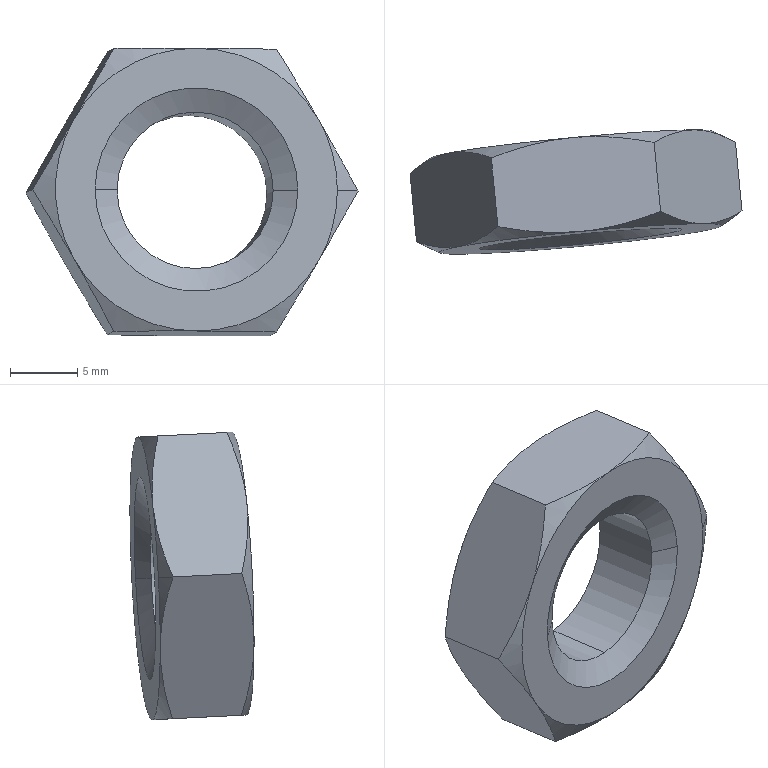Part | SolidWorks | features BaseBody 1 | 1 solid | 28 faces | box 24.623 x 9.204 x 21.336 mm | volume 1841 mm3 | cone 18 | plane 8 | cylinder 2 | commonest cylinder face diameters 11.62 x2
STEP:
#1=CARTESIAN_POINT('',(1944.046,536.426,848.503));
#2=VERTEX_POINT('',#1);
#3=CARTESIAN_POINT('',(1945.447,536.291,843.253));
#4=VERTEX_POINT('',#3);
#5=CARTESIAN_POINT('',(1934.993,535.304,843.303));
#6=DIRECTION('',(-0.09408,0.9943,-0.05066));
#7=DIRECTION('',(0.8622,0.1068,0.4952));
#8=AXIS2_PLACEMENT_3D('',#5,#6,#7);
#9=CIRCLE('',#8,10.5);
#10=EDGE_CURVE('',#2,#4,#9,.T.);
#11=ORIENTED_EDGE('',*,*,#10,.T.);
#12=CARTESIAN_POINT('',(1946.976,537.376,843.198));
#13=VERTEX_POINT('',#12);
#14=CARTESIAN_POINT('',(1946.211,536.833,843.226));
#15=DIRECTION('',(0.8151,0.5785,-0.02947));
#16=VECTOR('',#15,1000.);
#17=LINE('',#14,#16);
#18=EDGE_CURVE('',#4,#13,#17,.T.);
#19=ORIENTED_EDGE('',*,*,#18,.T.);
#20=CARTESIAN_POINT('',(1944.046,536.426,848.503));
#21=CARTESIAN_POINT('',(1944.561,536.429,847.606));
#22=CARTESIAN_POINT('',(1945.061,536.521,846.716));
#23=CARTESIAN_POINT('',(1946.035,536.851,844.949));
#24=CARTESIAN_POINT('',(1946.51,537.089,844.071));
#25=CARTESIAN_POINT('',(1946.976,537.376,843.198));
#26=B_SPLINE_CURVE_WITH_KNOTS('',3,(#20,#21,#22,#23,#24,#25),.UNSPECIFIED.,.F.,.F.,(4,2,4),(0.,0.003067,0.006134),.UNSPECIFIED.);
#27=EDGE_CURVE('',#2,#13,#26,.T.);
#28=ORIENTED_EDGE('',*,*,#27,.F.);
#29=EDGE_LOOP('',(#11,#19,#28));
#30=FACE_OUTER_BOUND('',#29,.T.);
#31=CARTESIAN_POINT('',(1934.949,535.77,843.28));
#32=DIRECTION('',(-0.09408,0.9943,-0.05066));
#33=DIRECTION('',(0.9956,0.09396,-0.004782));
#34=AXIS2_PLACEMENT_3D('',#31,#32,#33);
#35=CONICAL_SURFACE('',#34,11.312,1.047);
#36=ADVANCED_FACE('',(#30),#35,.T.);
#37=CARTESIAN_POINT('',(1925.282,541.677,848.235));
#38=VERTEX_POINT('',#37);
#39=CARTESIAN_POINT('',(1923.881,541.278,842.999));
#40=VERTEX_POINT('',#39);
#41=CARTESIAN_POINT('',(1934.335,542.264,842.949));
#42=DIRECTION('',(0.09408,-0.9943,0.05066));
#43=DIRECTION('',(-0.8622,-0.05593,0.5035));
#44=AXIS2_PLACEMENT_3D('',#41,#42,#43);
#45=CIRCLE('',#44,10.5);
#46=EDGE_CURVE('',#38,#40,#45,.T.);
#47=ORIENTED_EDGE('',*,*,#46,.T.);
#48=CARTESIAN_POINT('',(1922.352,540.193,843.054));
#49=VERTEX_POINT('',#48);
#50=CARTESIAN_POINT('',(1923.117,540.735,843.027));
#51=DIRECTION('',(-0.8151,-0.5785,0.02947));
#52=VECTOR('',#51,1000.);
#53=LINE('',#50,#52);
#54=EDGE_CURVE('',#40,#49,#53,.T.);
#55=ORIENTED_EDGE('',*,*,#54,.T.);
#56=CARTESIAN_POINT('',(1922.352,540.193,843.054));
#57=CARTESIAN_POINT('',(1922.818,540.567,843.894));
#58=CARTESIAN_POINT('',(1923.293,540.892,844.743));
#59=CARTESIAN_POINT('',(1924.267,541.401,846.467));
#60=CARTESIAN_POINT('',(1924.767,541.583,847.343));
#61=CARTESIAN_POINT('',(1925.282,541.677,848.235));
#62=B_SPLINE_CURVE_WITH_KNOTS('',3,(#56,#57,#58,#59,#60,#61),.UNSPECIFIED.,.F.,.F.,(4,2,4),(0.,0.003067,0.006134),.UNSPECIFIED.);
#63=EDGE_CURVE('',#49,#38,#62,.T.);
#64=ORIENTED_EDGE('',*,*,#63,.T.);
#65=EDGE_LOOP('',(#47,#55,#64));
#66=FACE_OUTER_BOUND('',#65,.T.);
#67=CARTESIAN_POINT('',(1934.379,541.798,842.973));
#68=DIRECTION('',(0.09408,-0.9943,0.05066));
#69=DIRECTION('',(-0.9956,-0.09396,0.004782));
#70=AXIS2_PLACEMENT_3D('',#67,#68,#69);
#71=CONICAL_SURFACE('',#70,11.312,1.047);
#72=ADVANCED_FACE('',(#66),#71,.T.);
#73=CARTESIAN_POINT('',(1934.335,542.798,853.435));
#74=VERTEX_POINT('',#73);
#75=CARTESIAN_POINT('',(1943.388,543.386,848.148));
#76=VERTEX_POINT('',#75);
#77=CARTESIAN_POINT('',(1934.335,542.264,842.949));
#78=DIRECTION('',(-0.09408,0.9943,-0.05066));
#79=DIRECTION('',(-0.000005848,0.05089,0.9987));
#80=AXIS2_PLACEMENT_3D('',#77,#78,#79);
#81=CIRCLE('',#80,10.5);
#82=EDGE_CURVE('',#74,#76,#81,.T.);
#83=ORIENTED_EDGE('',*,*,#82,.T.);
#84=CARTESIAN_POINT('',(1943.388,542.851,837.662));
#85=VERTEX_POINT('',#84);
#86=CARTESIAN_POINT('',(1934.335,542.264,842.949));
#87=DIRECTION('',(0.09408,-0.9943,0.05066));
#88=DIRECTION('',(0.8622,0.05593,-0.5035));
#89=AXIS2_PLACEMENT_3D('',#86,#87,#88);
#90=CIRCLE('',#89,10.5);
#91=EDGE_CURVE('',#85,#76,#90,.T.);
#92=ORIENTED_EDGE('',*,*,#91,.F.);
#93=CARTESIAN_POINT('',(1934.335,541.73,832.462));
#94=VERTEX_POINT('',#93);
#95=CARTESIAN_POINT('',(1934.335,542.264,842.949));
#96=DIRECTION('',(-0.09408,0.9943,-0.05066));
#97=DIRECTION('',(0.8622,0.05593,-0.5035));
#98=AXIS2_PLACEMENT_3D('',#95,#96,#97);
#99=CIRCLE('',#98,10.5);
#100=EDGE_CURVE('',#85,#94,#99,.T.);
#101=ORIENTED_EDGE('',*,*,#100,.T.);
#102=CARTESIAN_POINT('',(1925.282,541.143,837.749));
#103=VERTEX_POINT('',#102);
#104=CARTESIAN_POINT('',(1934.335,542.264,842.949));
#105=DIRECTION('',(-0.09408,0.9943,-0.05066));
#106=DIRECTION('',(0.000005848,-0.05089,-0.9987));
#107=AXIS2_PLACEMENT_3D('',#104,#105,#106);
#108=CIRCLE('',#107,10.5);
#109=EDGE_CURVE('',#94,#103,#108,.T.);
#110=ORIENTED_EDGE('',*,*,#109,.T.);
#111=CARTESIAN_POINT('',(1934.335,542.264,842.949));
#112=DIRECTION('',(0.09408,-0.9943,0.05066));
#113=DIRECTION('',(-0.8622,-0.05593,0.5035));
#114=AXIS2_PLACEMENT_3D('',#111,#112,#113);
#115=CIRCLE('',#114,10.5);
#116=EDGE_CURVE('',#40,#103,#115,.T.);
#117=ORIENTED_EDGE('',*,*,#116,.F.);
#118=ORIENTED_EDGE('',*,*,#46,.F.);
#119=CARTESIAN_POINT('',(1934.335,542.264,842.949));
#120=DIRECTION('',(-0.09408,0.9943,-0.05066));
#121=DIRECTION('',(-0.8622,-0.05593,0.5035));
#122=AXIS2_PLACEMENT_3D('',#119,#120,#121);
#123=CIRCLE('',#122,10.5);
#124=EDGE_CURVE('',#38,#74,#123,.T.);
#125=ORIENTED_EDGE('',*,*,#124,.T.);
#126=EDGE_LOOP('',(#83,#92,#101,#110,#117,#118,#125));
#127=FACE_OUTER_BOUND('',#126,.T.);
#128=CARTESIAN_POINT('',(1941.851,542.974,842.913));
#129=VERTEX_POINT('',#128);
#130=CARTESIAN_POINT('',(1926.818,541.555,842.985));
#131=VERTEX_POINT('',#130);
#132=CARTESIAN_POINT('',(1934.335,542.264,842.949));
#133=DIRECTION('',(0.09408,-0.9943,0.05066));
#134=DIRECTION('',(0.9956,0.09396,-0.004782));
#135=AXIS2_PLACEMENT_3D('',#132,#133,#134);
#136=CIRCLE('',#135,7.55);
#137=EDGE_CURVE('',#129,#131,#136,.T.);
#138=ORIENTED_EDGE('',*,*,#137,.T.);
#139=CARTESIAN_POINT('',(1934.335,542.264,842.949));
#140=DIRECTION('',(0.09408,-0.9943,0.05066));
#141=DIRECTION('',(-0.9956,-0.09396,0.004782));
#142=AXIS2_PLACEMENT_3D('',#139,#140,#141);
#143=CIRCLE('',#142,7.55);
#144=EDGE_CURVE('',#131,#129,#143,.T.);
#145=ORIENTED_EDGE('',*,*,#144,.T.);
#146=EDGE_LOOP('',(#138,#145));
#147=FACE_BOUND('',#146,.T.);
#148=CARTESIAN_POINT('',(1934.335,542.264,842.949));
#149=DIRECTION('',(0.09408,-0.9943,0.05066));
#150=DIRECTION('',(0.000005848,-0.05089,-0.9987));
#151=AXIS2_PLACEMENT_3D('',#148,#149,#150);
#152=PLANE('',#151);
#153=ADVANCED_FACE('',(#127,#147),#152,.F.);
#154=CARTESIAN_POINT('',(1928.388,540.228,832.539));
#155=VERTEX_POINT('',#154);
#156=CARTESIAN_POINT('',(1928.388,540.228,832.539));
#157=CARTESIAN_POINT('',(1927.868,540.509,833.383));
#158=CARTESIAN_POINT('',(1927.349,540.741,834.237));
#159=CARTESIAN_POINT('',(1926.313,541.059,835.971));
#160=CARTESIAN_POINT('',(1925.797,541.146,836.852));
#161=CARTESIAN_POINT('',(1925.282,541.143,837.749));
#162=B_SPLINE_CURVE_WITH_KNOTS('',3,(#156,#157,#158,#159,#160,#161),.UNSPECIFIED.,.F.,.F.,(4,2,4),(0.,0.003067,0.006134),.UNSPECIFIED.);
#163=EDGE_CURVE('',#155,#103,#162,.T.);
#164=ORIENTED_EDGE('',*,*,#163,.T.);
#165=ORIENTED_EDGE('',*,*,#109,.F.);
#166=CARTESIAN_POINT('',(1934.335,541.73,832.462));
#167=CARTESIAN_POINT('',(1933.305,541.633,832.467));
#168=CARTESIAN_POINT('',(1932.297,541.448,832.477));
#169=CARTESIAN_POINT('',(1930.318,540.933,832.503));
#170=CARTESIAN_POINT('',(1929.347,540.605,832.52));
#171=CARTESIAN_POINT('',(1928.388,540.228,832.539));
#172=B_SPLINE_CURVE_WITH_KNOTS('',3,(#166,#167,#168,#169,#170,#171),.UNSPECIFIED.,.F.,.F.,(4,2,4),(0.,0.003067,0.006134),.UNSPECIFIED.);
#173=EDGE_CURVE('',#94,#155,#172,.T.);
#174=ORIENTED_EDGE('',*,*,#173,.T.);
#175=EDGE_LOOP('',(#164,#165,#174));
#176=FACE_OUTER_BOUND('',#175,.T.);
#177=CARTESIAN_POINT('',(1934.379,541.798,842.973));
#178=DIRECTION('',(0.09408,-0.9943,0.05066));
#179=DIRECTION('',(-0.9956,-0.09396,0.004782));
#180=AXIS2_PLACEMENT_3D('',#177,#178,#179);
#181=CONICAL_SURFACE('',#180,11.312,1.047);
#182=ADVANCED_FACE('',(#176),#181,.T.);
#183=CARTESIAN_POINT('',(1940.458,541.367,832.481));
#184=VERTEX_POINT('',#183);
#185=CARTESIAN_POINT('',(1940.458,541.367,832.481));
#186=CARTESIAN_POINT('',(1939.445,541.558,832.471));
#187=CARTESIAN_POINT('',(1938.43,541.699,832.464));
#188=CARTESIAN_POINT('',(1936.389,541.834,832.457));
#189=CARTESIAN_POINT('',(1935.365,541.827,832.457));
#190=CARTESIAN_POINT('',(1934.335,541.73,832.462));
#191=B_SPLINE_CURVE_WITH_KNOTS('',3,(#185,#186,#187,#188,#189,#190),.UNSPECIFIED.,.F.,.F.,(4,2,4),(0.,0.003067,0.006134),.UNSPECIFIED.);
#192=EDGE_CURVE('',#184,#94,#191,.T.);
#193=ORIENTED_EDGE('',*,*,#192,.T.);
#194=ORIENTED_EDGE('',*,*,#100,.F.);
#195=CARTESIAN_POINT('',(1943.388,542.851,837.662));
#196=CARTESIAN_POINT('',(1942.873,542.757,836.77));
#197=CARTESIAN_POINT('',(1942.373,542.575,835.894));
#198=CARTESIAN_POINT('',(1941.399,542.067,834.169));
#199=CARTESIAN_POINT('',(1940.924,541.741,833.321));
#200=CARTESIAN_POINT('',(1940.458,541.367,832.481));
#201=B_SPLINE_CURVE_WITH_KNOTS('',3,(#195,#196,#197,#198,#199,#200),.UNSPECIFIED.,.F.,.F.,(4,2,4),(0.,0.003067,0.006134),.UNSPECIFIED.);
#202=EDGE_CURVE('',#85,#184,#201,.T.);
#203=ORIENTED_EDGE('',*,*,#202,.T.);
#204=EDGE_LOOP('',(#193,#194,#203));
#205=FACE_OUTER_BOUND('',#204,.T.);
#206=CARTESIAN_POINT('',(1934.379,541.798,842.973));
#207=DIRECTION('',(0.09408,-0.9943,0.05066));
#208=DIRECTION('',(-0.9956,-0.09396,0.004782));
#209=AXIS2_PLACEMENT_3D('',#206,#207,#208);
#210=CONICAL_SURFACE('',#209,11.312,1.047);
#211=ADVANCED_FACE('',(#205),#210,.T.);
#212=CARTESIAN_POINT('',(1928.388,541.296,853.512));
#213=VERTEX_POINT('',#212);
#214=CARTESIAN_POINT('',(1928.388,541.296,853.512));
#215=CARTESIAN_POINT('',(1929.347,541.674,853.492));
#216=CARTESIAN_POINT('',(1930.318,542.002,853.476));
#217=CARTESIAN_POINT('',(1932.297,542.516,853.45));
#218=CARTESIAN_POINT('',(1933.305,542.701,853.44));
#219=CARTESIAN_POINT('',(1934.335,542.798,853.435));
#220=B_SPLINE_CURVE_WITH_KNOTS('',3,(#214,#215,#216,#217,#218,#219),.UNSPECIFIED.,.F.,.F.,(4,2,4),(0.,0.003067,0.006134),.UNSPECIFIED.);
#221=EDGE_CURVE('',#213,#74,#220,.T.);
#222=ORIENTED_EDGE('',*,*,#221,.T.);
#223=ORIENTED_EDGE('',*,*,#124,.F.);
#224=CARTESIAN_POINT('',(1925.282,541.677,848.235));
#225=CARTESIAN_POINT('',(1925.797,541.771,849.128));
#226=CARTESIAN_POINT('',(1926.313,541.775,850.013));
#227=CARTESIAN_POINT('',(1927.349,541.634,851.77));
#228=CARTESIAN_POINT('',(1927.868,541.49,852.643));
#229=CARTESIAN_POINT('',(1928.388,541.296,853.512));
#230=B_SPLINE_CURVE_WITH_KNOTS('',3,(#224,#225,#226,#227,#228,#229),.UNSPECIFIED.,.F.,.F.,(4,2,4),(0.,0.003067,0.006134),.UNSPECIFIED.);
#231=EDGE_CURVE('',#38,#213,#230,.T.);
#232=ORIENTED_EDGE('',*,*,#231,.T.);
#233=EDGE_LOOP('',(#222,#223,#232));
#234=FACE_OUTER_BOUND('',#233,.T.);
#235=CARTESIAN_POINT('',(1934.379,541.798,842.973));
#236=DIRECTION('',(0.09408,-0.9943,0.05066));
#237=DIRECTION('',(-0.9956,-0.09396,0.004782));
#238=AXIS2_PLACEMENT_3D('',#235,#236,#237);
#239=CONICAL_SURFACE('',#238,11.312,1.047);
#240=ADVANCED_FACE('',(#234),#239,.T.);
#241=CARTESIAN_POINT('',(1940.458,542.436,853.454));
#242=VERTEX_POINT('',#241);
#243=CARTESIAN_POINT('',(1940.458,542.436,853.454));
#244=CARTESIAN_POINT('',(1940.924,542.723,852.58));
#245=CARTESIAN_POINT('',(1941.399,542.96,851.703));
#246=CARTESIAN_POINT('',(1942.373,543.291,849.936));
#247=CARTESIAN_POINT('',(1942.873,543.383,849.046));
#248=CARTESIAN_POINT('',(1943.388,543.386,848.148));
#249=B_SPLINE_CURVE_WITH_KNOTS('',3,(#243,#244,#245,#246,#247,#248),.UNSPECIFIED.,.F.,.F.,(4,2,4),(0.,0.003067,0.006134),.UNSPECIFIED.);
#250=EDGE_CURVE('',#242,#76,#249,.T.);
#251=ORIENTED_EDGE('',*,*,#250,.T.);
#252=ORIENTED_EDGE('',*,*,#82,.F.);
#253=CARTESIAN_POINT('',(1934.335,542.798,853.435));
#254=CARTESIAN_POINT('',(1935.365,542.896,853.43));
#255=CARTESIAN_POINT('',(1936.389,542.902,853.43));
#256=CARTESIAN_POINT('',(1938.429,542.767,853.437));
#257=CARTESIAN_POINT('',(1939.445,542.627,853.444));
#258=CARTESIAN_POINT('',(1940.458,542.436,853.454));
#259=B_SPLINE_CURVE_WITH_KNOTS('',3,(#253,#254,#255,#256,#257,#258),.UNSPECIFIED.,.F.,.F.,(4,2,4),(0.,0.003067,0.006134),.UNSPECIFIED.);
#260=EDGE_CURVE('',#74,#242,#259,.T.);
#261=ORIENTED_EDGE('',*,*,#260,.T.);
#262=EDGE_LOOP('',(#251,#252,#261));
#263=FACE_OUTER_BOUND('',#262,.T.);
#264=CARTESIAN_POINT('',(1934.379,541.798,842.973));
#265=DIRECTION('',(0.09408,-0.9943,0.05066));
#266=DIRECTION('',(-0.9956,-0.09396,0.004782));
#267=AXIS2_PLACEMENT_3D('',#264,#265,#266);
#268=CONICAL_SURFACE('',#267,11.312,1.047);
#269=ADVANCED_FACE('',(#263),#268,.T.);
#270=ORIENTED_EDGE('',*,*,#91,.T.);
#271=CARTESIAN_POINT('',(1946.493,542.471,842.938));
#272=VERTEX_POINT('',#271);
#273=CARTESIAN_POINT('',(1943.388,543.386,848.148));
#274=CARTESIAN_POINT('',(1943.903,543.389,847.251));
#275=CARTESIAN_POINT('',(1944.419,543.303,846.371));
#276=CARTESIAN_POINT('',(1945.455,542.984,844.636));
#277=CARTESIAN_POINT('',(1945.974,542.752,843.783));
#278=CARTESIAN_POINT('',(1946.493,542.471,842.938));
#279=B_SPLINE_CURVE_WITH_KNOTS('',3,(#273,#274,#275,#276,#277,#278),.UNSPECIFIED.,.F.,.F.,(4,2,4),(0.,0.003067,0.006134),.UNSPECIFIED.);
#280=EDGE_CURVE('',#76,#272,#279,.T.);
#281=ORIENTED_EDGE('',*,*,#280,.T.);
#282=CARTESIAN_POINT('',(1946.493,542.471,842.938));
#283=CARTESIAN_POINT('',(1945.974,542.665,842.07));
#284=CARTESIAN_POINT('',(1945.455,542.808,841.197));
#285=CARTESIAN_POINT('',(1944.419,542.949,839.439));
#286=CARTESIAN_POINT('',(1943.903,542.946,838.554));
#287=CARTESIAN_POINT('',(1943.388,542.851,837.662));
#288=B_SPLINE_CURVE_WITH_KNOTS('',3,(#282,#283,#284,#285,#286,#287),.UNSPECIFIED.,.F.,.F.,(4,2,4),(0.,0.003067,0.006134),.UNSPECIFIED.);
#289=EDGE_CURVE('',#272,#85,#288,.T.);
#290=ORIENTED_EDGE('',*,*,#289,.T.);
#291=EDGE_LOOP('',(#270,#281,#290));
#292=FACE_OUTER_BOUND('',#291,.T.);
#293=CARTESIAN_POINT('',(1934.379,541.798,842.973));
#294=DIRECTION('',(0.09408,-0.9943,0.05066));
#295=DIRECTION('',(-0.9956,-0.09396,0.004782));
#296=AXIS2_PLACEMENT_3D('',#293,#294,#295);
#297=CONICAL_SURFACE('',#296,11.312,1.047);
#298=ADVANCED_FACE('',(#292),#297,.T.);
#299=ORIENTED_EDGE('',*,*,#173,.F.);
#300=ORIENTED_EDGE('',*,*,#192,.F.);
#301=CARTESIAN_POINT('',(1940.94,536.272,832.741));
#302=VERTEX_POINT('',#301);
#303=CARTESIAN_POINT('',(1940.458,541.367,832.481));
#304=DIRECTION('',(0.09408,-0.9943,0.05066));
#305=VECTOR('',#304,1000.);
#306=LINE('',#303,#305);
#307=EDGE_CURVE('',#184,#302,#306,.T.);
#308=ORIENTED_EDGE('',*,*,#307,.T.);
#309=CARTESIAN_POINT('',(1934.993,534.77,832.817));
#310=VERTEX_POINT('',#309);
#311=CARTESIAN_POINT('',(1940.94,536.272,832.741));
#312=CARTESIAN_POINT('',(1939.981,535.895,832.76));
#313=CARTESIAN_POINT('',(1939.01,535.566,832.776));
#314=CARTESIAN_POINT('',(1937.031,535.052,832.803));
#315=CARTESIAN_POINT('',(1936.023,534.867,832.812));
#316=CARTESIAN_POINT('',(1934.993,534.77,832.817));
#317=B_SPLINE_CURVE_WITH_KNOTS('',3,(#311,#312,#313,#314,#315,#316),.UNSPECIFIED.,.F.,.F.,(4,2,4),(0.,0.003067,0.006134),.UNSPECIFIED.);
#318=EDGE_CURVE('',#302,#310,#317,.T.);
#319=ORIENTED_EDGE('',*,*,#318,.T.);
#320=CARTESIAN_POINT('',(1928.87,535.133,832.798));
#321=VERTEX_POINT('',#320);
#322=CARTESIAN_POINT('',(1934.993,534.77,832.817));
#323=CARTESIAN_POINT('',(1933.963,534.673,832.822));
#324=CARTESIAN_POINT('',(1932.939,534.666,832.822));
#325=CARTESIAN_POINT('',(1930.898,534.801,832.815));
#326=CARTESIAN_POINT('',(1929.883,534.942,832.808));
#327=CARTESIAN_POINT('',(1928.87,535.133,832.798));
#328=B_SPLINE_CURVE_WITH_KNOTS('',3,(#322,#323,#324,#325,#326,#327),.UNSPECIFIED.,.F.,.F.,(4,2,4),(0.,0.003067,0.006134),.UNSPECIFIED.);
#329=EDGE_CURVE('',#310,#321,#328,.T.);
#330=ORIENTED_EDGE('',*,*,#329,.T.);
#331=CARTESIAN_POINT('',(1928.388,540.228,832.539));
#332=DIRECTION('',(0.09408,-0.9943,0.05066));
#333=VECTOR('',#332,1000.);
#334=LINE('',#331,#333);
#335=EDGE_CURVE('',#155,#321,#334,.T.);
#336=ORIENTED_EDGE('',*,*,#335,.F.);
#337=EDGE_LOOP('',(#299,#300,#308,#319,#330,#336));
#338=FACE_OUTER_BOUND('',#337,.T.);
#339=CARTESIAN_POINT('',(1940.37,542.299,832.433));
#340=DIRECTION('',(0.000005848,-0.05089,-0.9987));
#341=DIRECTION('',(0.9956,0.09396,-0.004782));
#342=AXIS2_PLACEMENT_3D('',#339,#340,#341);
#343=PLANE('',#342);
#344=ADVANCED_FACE('',(#338),#343,.T.);
#345=ORIENTED_EDGE('',*,*,#202,.F.);
#346=ORIENTED_EDGE('',*,*,#289,.F.);
#347=CARTESIAN_POINT('',(1946.493,542.471,842.938));
#348=DIRECTION('',(0.09408,-0.9943,0.05066));
#349=VECTOR('',#348,1000.);
#350=LINE('',#347,#349);
#351=EDGE_CURVE('',#272,#13,#350,.T.);
#352=ORIENTED_EDGE('',*,*,#351,.T.);
#353=CARTESIAN_POINT('',(1944.046,535.891,838.017));
#354=VERTEX_POINT('',#353);
#355=CARTESIAN_POINT('',(1946.976,537.376,843.198));
#356=CARTESIAN_POINT('',(1946.51,537.001,842.358));
#357=CARTESIAN_POINT('',(1946.035,536.676,841.509));
#358=CARTESIAN_POINT('',(1945.061,536.168,839.785));
#359=CARTESIAN_POINT('',(1944.561,535.986,838.909));
#360=CARTESIAN_POINT('',(1944.046,535.891,838.017));
#361=B_SPLINE_CURVE_WITH_KNOTS('',3,(#355,#356,#357,#358,#359,#360),.UNSPECIFIED.,.F.,.F.,(4,2,4),(0.,0.003067,0.006134),.UNSPECIFIED.);
#362=EDGE_CURVE('',#13,#354,#361,.T.);
#363=ORIENTED_EDGE('',*,*,#362,.T.);
#364=CARTESIAN_POINT('',(1944.046,535.891,838.017));
#365=CARTESIAN_POINT('',(1943.531,535.797,837.124));
#366=CARTESIAN_POINT('',(1943.015,535.793,836.24));
#367=CARTESIAN_POINT('',(1941.979,535.934,834.482));
#368=CARTESIAN_POINT('',(1941.46,536.078,833.609));
#369=CARTESIAN_POINT('',(1940.94,536.272,832.741));
#370=B_SPLINE_CURVE_WITH_KNOTS('',3,(#364,#365,#366,#367,#368,#369),.UNSPECIFIED.,.F.,.F.,(4,2,4),(0.,0.003067,0.006134),.UNSPECIFIED.);
#371=EDGE_CURVE('',#354,#302,#370,.T.);
#372=ORIENTED_EDGE('',*,*,#371,.T.);
#373=ORIENTED_EDGE('',*,*,#307,.F.);
#374=EDGE_LOOP('',(#345,#346,#352,#363,#372,#373));
#375=FACE_OUTER_BOUND('',#374,.T.);
#376=CARTESIAN_POINT('',(1946.405,543.403,842.891));
#377=DIRECTION('',(0.8622,0.05593,-0.5035));
#378=DIRECTION('',(0.4978,0.09105,0.8625));
#379=AXIS2_PLACEMENT_3D('',#376,#377,#378);
#380=PLANE('',#379);
#381=ADVANCED_FACE('',(#375),#380,.T.);
#382=ORIENTED_EDGE('',*,*,#280,.F.);
#383=ORIENTED_EDGE('',*,*,#250,.F.);
#384=CARTESIAN_POINT('',(1940.94,537.341,853.713));
#385=VERTEX_POINT('',#384);
#386=CARTESIAN_POINT('',(1940.458,542.436,853.454));
#387=DIRECTION('',(0.09408,-0.9943,0.05066));
#388=VECTOR('',#387,1000.);
#389=LINE('',#386,#388);
#390=EDGE_CURVE('',#242,#385,#389,.T.);
#391=ORIENTED_EDGE('',*,*,#390,.T.);
#392=CARTESIAN_POINT('',(1940.94,537.341,853.713));
#393=CARTESIAN_POINT('',(1941.46,537.059,852.869));
#394=CARTESIAN_POINT('',(1941.979,536.828,852.015));
#395=CARTESIAN_POINT('',(1943.015,536.509,850.281));
#396=CARTESIAN_POINT('',(1943.531,536.423,849.4));
#397=CARTESIAN_POINT('',(1944.046,536.426,848.503));
#398=B_SPLINE_CURVE_WITH_KNOTS('',3,(#392,#393,#394,#395,#396,#397),.UNSPECIFIED.,.F.,.F.,(4,2,4),(0.,0.003067,0.006134),.UNSPECIFIED.);
#399=EDGE_CURVE('',#385,#2,#398,.T.);
#400=ORIENTED_EDGE('',*,*,#399,.T.);
#401=ORIENTED_EDGE('',*,*,#27,.T.);
#402=ORIENTED_EDGE('',*,*,#351,.F.);
#403=EDGE_LOOP('',(#382,#383,#391,#400,#401,#402));
#404=FACE_OUTER_BOUND('',#403,.T.);
#405=CARTESIAN_POINT('',(1940.37,543.368,853.406));
#406=DIRECTION('',(0.8622,0.1068,0.4952));
#407=DIRECTION('',(-0.4978,-0.00291,0.8673));
#408=AXIS2_PLACEMENT_3D('',#405,#406,#407);
#409=PLANE('',#408);
#410=ADVANCED_FACE('',(#404),#409,.T.);
#411=ORIENTED_EDGE('',*,*,#260,.F.);
#412=ORIENTED_EDGE('',*,*,#221,.F.);
#413=CARTESIAN_POINT('',(1928.87,536.201,853.771));
#414=VERTEX_POINT('',#413);
#415=CARTESIAN_POINT('',(1928.388,541.296,853.512));
#416=DIRECTION('',(0.09408,-0.9943,0.05066));
#417=VECTOR('',#416,1000.);
#418=LINE('',#415,#417);
#419=EDGE_CURVE('',#213,#414,#418,.T.);
#420=ORIENTED_EDGE('',*,*,#419,.T.);
#421=CARTESIAN_POINT('',(1934.993,535.839,853.79));
#422=VERTEX_POINT('',#421);
#423=CARTESIAN_POINT('',(1928.87,536.201,853.771));
#424=CARTESIAN_POINT('',(1929.882,536.01,853.781));
#425=CARTESIAN_POINT('',(1930.898,535.87,853.788));
#426=CARTESIAN_POINT('',(1932.939,535.735,853.795));
#427=CARTESIAN_POINT('',(1933.963,535.741,853.795));
#428=CARTESIAN_POINT('',(1934.993,535.839,853.79));
#429=B_SPLINE_CURVE_WITH_KNOTS('',3,(#423,#424,#425,#426,#427,#428),.UNSPECIFIED.,.F.,.F.,(4,2,4),(0.,0.003067,0.006134),.UNSPECIFIED.);
#430=EDGE_CURVE('',#414,#422,#429,.T.);
#431=ORIENTED_EDGE('',*,*,#430,.T.);
#432=CARTESIAN_POINT('',(1934.993,535.839,853.79));
#433=CARTESIAN_POINT('',(1936.023,535.936,853.785));
#434=CARTESIAN_POINT('',(1937.031,536.121,853.775));
#435=CARTESIAN_POINT('',(1939.01,536.635,853.749));
#436=CARTESIAN_POINT('',(1939.981,536.963,853.733));
#437=CARTESIAN_POINT('',(1940.94,537.341,853.713));
#438=B_SPLINE_CURVE_WITH_KNOTS('',3,(#432,#433,#434,#435,#436,#437),.UNSPECIFIED.,.F.,.F.,(4,2,4),(0.,0.003067,0.006134),.UNSPECIFIED.);
#439=EDGE_CURVE('',#422,#385,#438,.T.);
#440=ORIENTED_EDGE('',*,*,#439,.T.);
#441=ORIENTED_EDGE('',*,*,#390,.F.);
#442=EDGE_LOOP('',(#411,#412,#420,#431,#440,#441));
#443=FACE_OUTER_BOUND('',#442,.T.);
#444=CARTESIAN_POINT('',(1928.299,542.229,853.464));
#445=DIRECTION('',(-0.000005848,0.05089,0.9987));
#446=DIRECTION('',(-0.9956,-0.09396,0.004782));
#447=AXIS2_PLACEMENT_3D('',#444,#445,#446);
#448=PLANE('',#447);
#449=ADVANCED_FACE('',(#443),#448,.T.);
#450=ORIENTED_EDGE('',*,*,#231,.F.);
#451=ORIENTED_EDGE('',*,*,#63,.F.);
#452=CARTESIAN_POINT('',(1922.834,535.097,843.314));
#453=VERTEX_POINT('',#452);
#454=CARTESIAN_POINT('',(1922.352,540.193,843.054));
#455=DIRECTION('',(0.09408,-0.9943,0.05066));
#456=VECTOR('',#455,1000.);
#457=LINE('',#454,#456);
#458=EDGE_CURVE('',#49,#453,#457,.T.);
#459=ORIENTED_EDGE('',*,*,#458,.T.);
#460=CARTESIAN_POINT('',(1925.94,534.717,848.59));
#461=VERTEX_POINT('',#460);
#462=CARTESIAN_POINT('',(1922.834,535.097,843.314));
#463=CARTESIAN_POINT('',(1923.354,534.903,844.183));
#464=CARTESIAN_POINT('',(1923.873,534.76,845.055));
#465=CARTESIAN_POINT('',(1924.909,534.619,846.813));
#466=CARTESIAN_POINT('',(1925.425,534.623,847.698));
#467=CARTESIAN_POINT('',(1925.94,534.717,848.59));
#468=B_SPLINE_CURVE_WITH_KNOTS('',3,(#462,#463,#464,#465,#466,#467),.UNSPECIFIED.,.F.,.F.,(4,2,4),(0.,0.003067,0.006134),.UNSPECIFIED.);
#469=EDGE_CURVE('',#453,#461,#468,.T.);
#470=ORIENTED_EDGE('',*,*,#469,.T.);
#471=CARTESIAN_POINT('',(1925.94,534.717,848.59));
#472=CARTESIAN_POINT('',(1926.455,534.811,849.482));
#473=CARTESIAN_POINT('',(1926.955,534.993,850.358));
#474=CARTESIAN_POINT('',(1927.929,535.502,852.083));
#475=CARTESIAN_POINT('',(1928.404,535.827,852.932));
#476=CARTESIAN_POINT('',(1928.87,536.201,853.771));
#477=B_SPLINE_CURVE_WITH_KNOTS('',3,(#471,#472,#473,#474,#475,#476),.UNSPECIFIED.,.F.,.F.,(4,2,4),(0.,0.003067,0.006134),.UNSPECIFIED.);
#478=EDGE_CURVE('',#461,#414,#477,.T.);
#479=ORIENTED_EDGE('',*,*,#478,.T.);
#480=ORIENTED_EDGE('',*,*,#419,.F.);
#481=EDGE_LOOP('',(#450,#451,#459,#470,#479,#480));
#482=FACE_OUTER_BOUND('',#481,.T.);
#483=CARTESIAN_POINT('',(1922.264,541.125,843.007));
#484=DIRECTION('',(-0.8622,-0.05593,0.5035));
#485=DIRECTION('',(-0.4978,-0.09105,-0.8625));
#486=AXIS2_PLACEMENT_3D('',#483,#484,#485);
#487=PLANE('',#486);
#488=ADVANCED_FACE('',(#482),#487,.T.);
#489=ORIENTED_EDGE('',*,*,#54,.F.);
#490=ORIENTED_EDGE('',*,*,#116,.T.);
#491=CARTESIAN_POINT('',(1925.282,541.143,837.749));
#492=CARTESIAN_POINT('',(1924.767,541.14,838.646));
#493=CARTESIAN_POINT('',(1924.267,541.047,839.536));
#494=CARTESIAN_POINT('',(1923.293,540.717,841.303));
#495=CARTESIAN_POINT('',(1922.818,540.48,842.181));
#496=CARTESIAN_POINT('',(1922.352,540.193,843.054));
#497=B_SPLINE_CURVE_WITH_KNOTS('',3,(#491,#492,#493,#494,#495,#496),.UNSPECIFIED.,.F.,.F.,(4,2,4),(0.,0.003067,0.006134),.UNSPECIFIED.);
#498=EDGE_CURVE('',#103,#49,#497,.T.);
#499=ORIENTED_EDGE('',*,*,#498,.T.);
#500=EDGE_LOOP('',(#489,#490,#499));
#501=FACE_OUTER_BOUND('',#500,.T.);
#502=CARTESIAN_POINT('',(1934.379,541.798,842.973));
#503=DIRECTION('',(0.09408,-0.9943,0.05066));
#504=DIRECTION('',(-0.9956,-0.09396,0.004782));
#505=AXIS2_PLACEMENT_3D('',#502,#503,#504);
#506=CONICAL_SURFACE('',#505,11.312,1.047);
#507=ADVANCED_FACE('',(#501),#506,.T.);
#508=ORIENTED_EDGE('',*,*,#498,.F.);
#509=ORIENTED_EDGE('',*,*,#163,.F.);
#510=ORIENTED_EDGE('',*,*,#335,.T.);
#511=CARTESIAN_POINT('',(1925.94,534.183,838.104));
#512=VERTEX_POINT('',#511);
#513=CARTESIAN_POINT('',(1928.87,535.133,832.798));
#514=CARTESIAN_POINT('',(1928.404,534.846,833.672));
#515=CARTESIAN_POINT('',(1927.929,534.608,834.549));
#516=CARTESIAN_POINT('',(1926.955,534.278,836.317));
#517=CARTESIAN_POINT('',(1926.455,534.186,837.206));
#518=CARTESIAN_POINT('',(1925.94,534.183,838.104));
#519=B_SPLINE_CURVE_WITH_KNOTS('',3,(#513,#514,#515,#516,#517,#518),.UNSPECIFIED.,.F.,.F.,(4,2,4),(0.,0.003067,0.006134),.UNSPECIFIED.);
#520=EDGE_CURVE('',#321,#512,#519,.T.);
#521=ORIENTED_EDGE('',*,*,#520,.T.);
#522=CARTESIAN_POINT('',(1925.94,534.183,838.104));
#523=CARTESIAN_POINT('',(1925.425,534.18,839.001));
#524=CARTESIAN_POINT('',(1924.909,534.266,839.882));
#525=CARTESIAN_POINT('',(1923.873,534.585,841.616));
#526=CARTESIAN_POINT('',(1923.354,534.816,842.469));
#527=CARTESIAN_POINT('',(1922.834,535.097,843.314));
#528=B_SPLINE_CURVE_WITH_KNOTS('',3,(#522,#523,#524,#525,#526,#527),.UNSPECIFIED.,.F.,.F.,(4,2,4),(0.,0.003067,0.006134),.UNSPECIFIED.);
#529=EDGE_CURVE('',#512,#453,#528,.T.);
#530=ORIENTED_EDGE('',*,*,#529,.T.);
#531=ORIENTED_EDGE('',*,*,#458,.F.);
#532=EDGE_LOOP('',(#508,#509,#510,#521,#530,#531));
#533=FACE_OUTER_BOUND('',#532,.T.);
#534=CARTESIAN_POINT('',(1928.299,541.16,832.491));
#535=DIRECTION('',(-0.8622,-0.1068,-0.4952));
#536=DIRECTION('',(0.4978,0.00291,-0.8673));
#537=AXIS2_PLACEMENT_3D('',#534,#535,#536);
#538=PLANE('',#537);
#539=ADVANCED_FACE('',(#533),#538,.T.);
#540=ORIENTED_EDGE('',*,*,#329,.F.);
#541=CARTESIAN_POINT('',(1934.993,535.304,843.303));
#542=DIRECTION('',(-0.09408,0.9943,-0.05066));
#543=DIRECTION('',(0.000005848,-0.05089,-0.9987));
#544=AXIS2_PLACEMENT_3D('',#541,#542,#543);
#545=CIRCLE('',#544,10.5);
#546=EDGE_CURVE('',#310,#512,#545,.T.);
#547=ORIENTED_EDGE('',*,*,#546,.T.);
#548=ORIENTED_EDGE('',*,*,#520,.F.);
#549=EDGE_LOOP('',(#540,#547,#548));
#550=FACE_OUTER_BOUND('',#549,.T.);
#551=CARTESIAN_POINT('',(1934.949,535.77,843.28));
#552=DIRECTION('',(-0.09408,0.9943,-0.05066));
#553=DIRECTION('',(0.9956,0.09396,-0.004782));
#554=AXIS2_PLACEMENT_3D('',#551,#552,#553);
#555=CONICAL_SURFACE('',#554,11.312,1.047);
#556=ADVANCED_FACE('',(#550),#555,.T.);
#557=ORIENTED_EDGE('',*,*,#371,.F.);
#558=CARTESIAN_POINT('',(1934.993,535.304,843.303));
#559=DIRECTION('',(-0.09408,0.9943,-0.05066));
#560=DIRECTION('',(0.8622,0.05593,-0.5035));
#561=AXIS2_PLACEMENT_3D('',#558,#559,#560);
#562=CIRCLE('',#561,10.5);
#563=EDGE_CURVE('',#354,#310,#562,.T.);
#564=ORIENTED_EDGE('',*,*,#563,.T.);
#565=ORIENTED_EDGE('',*,*,#318,.F.);
#566=EDGE_LOOP('',(#557,#564,#565));
#567=FACE_OUTER_BOUND('',#566,.T.);
#568=CARTESIAN_POINT('',(1934.949,535.77,843.28));
#569=DIRECTION('',(-0.09408,0.9943,-0.05066));
#570=DIRECTION('',(0.9956,0.09396,-0.004782));
#571=AXIS2_PLACEMENT_3D('',#568,#569,#570);
#572=CONICAL_SURFACE('',#571,11.312,1.047);
#573=ADVANCED_FACE('',(#567),#572,.T.);
#574=ORIENTED_EDGE('',*,*,#478,.F.);
#575=CARTESIAN_POINT('',(1934.993,535.304,843.303));
#576=DIRECTION('',(-0.09408,0.9943,-0.05066));
#577=DIRECTION('',(-0.8622,-0.05593,0.5035));
#578=AXIS2_PLACEMENT_3D('',#575,#576,#577);
#579=CIRCLE('',#578,10.5);
#580=EDGE_CURVE('',#461,#422,#579,.T.);
#581=ORIENTED_EDGE('',*,*,#580,.T.);
#582=ORIENTED_EDGE('',*,*,#430,.F.);
#583=EDGE_LOOP('',(#574,#581,#582));
#584=FACE_OUTER_BOUND('',#583,.T.);
#585=CARTESIAN_POINT('',(1934.949,535.77,843.28));
#586=DIRECTION('',(-0.09408,0.9943,-0.05066));
#587=DIRECTION('',(0.9956,0.09396,-0.004782));
#588=AXIS2_PLACEMENT_3D('',#585,#586,#587);
#589=CONICAL_SURFACE('',#588,11.312,1.047);
#590=ADVANCED_FACE('',(#584),#589,.T.);
#591=ORIENTED_EDGE('',*,*,#439,.F.);
#592=CARTESIAN_POINT('',(1934.993,535.304,843.303));
#593=DIRECTION('',(-0.09408,0.9943,-0.05066));
#594=DIRECTION('',(-0.000005848,0.05089,0.9987));
#595=AXIS2_PLACEMENT_3D('',#592,#593,#594);
#596=CIRCLE('',#595,10.5);
#597=EDGE_CURVE('',#422,#2,#596,.T.);
#598=ORIENTED_EDGE('',*,*,#597,.T.);
#599=ORIENTED_EDGE('',*,*,#399,.F.);
#600=EDGE_LOOP('',(#591,#598,#599));
#601=FACE_OUTER_BOUND('',#600,.T.);
#602=CARTESIAN_POINT('',(1934.949,535.77,843.28));
#603=DIRECTION('',(-0.09408,0.9943,-0.05066));
#604=DIRECTION('',(0.9956,0.09396,-0.004782));
#605=AXIS2_PLACEMENT_3D('',#602,#603,#604);
#606=CONICAL_SURFACE('',#605,11.312,1.047);
#607=ADVANCED_FACE('',(#601),#606,.T.);
#608=ORIENTED_EDGE('',*,*,#18,.F.);
#609=CARTESIAN_POINT('',(1934.993,535.304,843.303));
#610=DIRECTION('',(-0.09408,0.9943,-0.05066));
#611=DIRECTION('',(0.8622,0.1068,0.4952));
#612=AXIS2_PLACEMENT_3D('',#609,#610,#611);
#613=CIRCLE('',#612,10.5);
#614=EDGE_CURVE('',#4,#354,#613,.T.);
#615=ORIENTED_EDGE('',*,*,#614,.T.);
#616=ORIENTED_EDGE('',*,*,#362,.F.);
#617=EDGE_LOOP('',(#608,#615,#616));
#618=FACE_OUTER_BOUND('',#617,.T.);
#619=CARTESIAN_POINT('',(1934.949,535.77,843.28));
#620=DIRECTION('',(-0.09408,0.9943,-0.05066));
#621=DIRECTION('',(0.9956,0.09396,-0.004782));
#622=AXIS2_PLACEMENT_3D('',#619,#620,#621);
#623=CONICAL_SURFACE('',#622,11.312,1.047);
#624=ADVANCED_FACE('',(#618),#623,.T.);
#625=ORIENTED_EDGE('',*,*,#563,.F.);
#626=ORIENTED_EDGE('',*,*,#614,.F.);
#627=ORIENTED_EDGE('',*,*,#10,.F.);
#628=ORIENTED_EDGE('',*,*,#597,.F.);
#629=ORIENTED_EDGE('',*,*,#580,.F.);
#630=CARTESIAN_POINT('',(1934.993,535.304,843.303));
#631=DIRECTION('',(-0.09408,0.9943,-0.05066));
#632=DIRECTION('',(-0.8622,-0.1068,-0.4952));
#633=AXIS2_PLACEMENT_3D('',#630,#631,#632);
#634=CIRCLE('',#633,10.5);
#635=EDGE_CURVE('',#512,#461,#634,.T.);
#636=ORIENTED_EDGE('',*,*,#635,.F.);
#637=ORIENTED_EDGE('',*,*,#546,.F.);
#638=EDGE_LOOP('',(#625,#626,#627,#628,#629,#636,#637));
#639=FACE_OUTER_BOUND('',#638,.T.);
#640=CARTESIAN_POINT('',(1942.51,536.014,843.267));
#641=VERTEX_POINT('',#640);
#642=CARTESIAN_POINT('',(1927.477,534.595,843.339));
#643=VERTEX_POINT('',#642);
#644=CARTESIAN_POINT('',(1934.993,535.304,843.303));
#645=DIRECTION('',(0.09408,-0.9943,0.05066));
#646=DIRECTION('',(0.9956,0.09396,-0.004782));
#647=AXIS2_PLACEMENT_3D('',#644,#645,#646);
#648=CIRCLE('',#647,7.55);
#649=EDGE_CURVE('',#641,#643,#648,.T.);
#650=ORIENTED_EDGE('',*,*,#649,.F.);
#651=CARTESIAN_POINT('',(1934.993,535.304,843.303));
#652=DIRECTION('',(0.09408,-0.9943,0.05066));
#653=DIRECTION('',(-0.9956,-0.09396,0.004782));
#654=AXIS2_PLACEMENT_3D('',#651,#652,#653);
#655=CIRCLE('',#654,7.55);
#656=EDGE_CURVE('',#643,#641,#655,.T.);
#657=ORIENTED_EDGE('',*,*,#656,.F.);
#658=EDGE_LOOP('',(#650,#657));
#659=FACE_BOUND('',#658,.T.);
#660=CARTESIAN_POINT('',(1934.993,535.304,843.303));
#661=DIRECTION('',(0.09408,-0.9943,0.05066));
#662=DIRECTION('',(0.000005848,-0.05089,-0.9987));
#663=AXIS2_PLACEMENT_3D('',#660,#661,#662);
#664=PLANE('',#663);
#665=ADVANCED_FACE('',(#639,#659),#664,.T.);
#666=ORIENTED_EDGE('',*,*,#529,.F.);
#667=ORIENTED_EDGE('',*,*,#635,.T.);
#668=ORIENTED_EDGE('',*,*,#469,.F.);
#669=EDGE_LOOP('',(#666,#667,#668));
#670=FACE_OUTER_BOUND('',#669,.T.);
#671=CARTESIAN_POINT('',(1934.949,535.77,843.28));
#672=DIRECTION('',(-0.09408,0.9943,-0.05066));
#673=DIRECTION('',(0.9956,0.09396,-0.004782));
#674=AXIS2_PLACEMENT_3D('',#671,#672,#673);
#675=CONICAL_SURFACE('',#674,11.312,1.047);
#676=ADVANCED_FACE('',(#670),#675,.T.);
#677=CARTESIAN_POINT('',(1929.114,535.757,843.28));
#678=VERTEX_POINT('',#677);
#679=CARTESIAN_POINT('',(1927.477,534.595,843.339));
#680=DIRECTION('',(-0.8151,-0.5785,0.02947));
#681=VECTOR('',#680,1000.);
#682=LINE('',#679,#681);
#683=EDGE_CURVE('',#678,#643,#682,.T.);
#684=ORIENTED_EDGE('',*,*,#683,.T.);
#685=ORIENTED_EDGE('',*,*,#656,.T.);
#686=CARTESIAN_POINT('',(1940.683,536.849,843.225));
#687=VERTEX_POINT('',#686);
#688=CARTESIAN_POINT('',(1942.51,536.014,843.267));
#689=DIRECTION('',(-0.9092,0.4158,-0.02119));
#690=VECTOR('',#689,1000.);
#691=LINE('',#688,#690);
#692=EDGE_CURVE('',#641,#687,#691,.T.);
#693=ORIENTED_EDGE('',*,*,#692,.T.);
#694=CARTESIAN_POINT('',(1934.899,536.007,837.45));
#695=VERTEX_POINT('',#694);
#696=CARTESIAN_POINT('',(1934.899,536.303,843.253));
#697=DIRECTION('',(-0.09408,0.9943,-0.05066));
#698=DIRECTION('',(0.9956,0.09396,-0.004782));
#699=AXIS2_PLACEMENT_3D('',#696,#697,#698);
#700=CIRCLE('',#699,5.81);
#701=EDGE_CURVE('',#687,#695,#700,.T.);
#702=ORIENTED_EDGE('',*,*,#701,.T.);
#703=CARTESIAN_POINT('',(1934.899,536.303,843.253));
#704=DIRECTION('',(-0.09408,0.9943,-0.05066));
#705=DIRECTION('',(0.000005848,-0.05089,-0.9987));
#706=AXIS2_PLACEMENT_3D('',#703,#704,#705);
#707=CIRCLE('',#706,5.81);
#708=EDGE_CURVE('',#695,#678,#707,.T.);
#709=ORIENTED_EDGE('',*,*,#708,.T.);
#710=EDGE_LOOP('',(#684,#685,#693,#702,#709));
#711=FACE_OUTER_BOUND('',#710,.T.);
#712=CARTESIAN_POINT('',(1934.946,535.804,843.278));
#713=DIRECTION('',(0.09408,-0.9943,0.05066));
#714=DIRECTION('',(-0.9956,-0.09396,0.004782));
#715=AXIS2_PLACEMENT_3D('',#712,#713,#714);
#716=CONICAL_SURFACE('',#715,6.68,1.047);
#717=ADVANCED_FACE('',(#711),#716,.F.);
#718=ORIENTED_EDGE('',*,*,#692,.F.);
#719=ORIENTED_EDGE('',*,*,#649,.T.);
#720=ORIENTED_EDGE('',*,*,#683,.F.);
#721=CARTESIAN_POINT('',(1934.899,536.599,849.055));
#722=VERTEX_POINT('',#721);
#723=CARTESIAN_POINT('',(1934.899,536.303,843.253));
#724=DIRECTION('',(-0.09408,0.9943,-0.05066));
#725=DIRECTION('',(-0.9956,-0.09396,0.004782));
#726=AXIS2_PLACEMENT_3D('',#723,#724,#725);
#727=CIRCLE('',#726,5.81);
#728=EDGE_CURVE('',#678,#722,#727,.T.);
#729=ORIENTED_EDGE('',*,*,#728,.T.);
#730=CARTESIAN_POINT('',(1934.899,536.303,843.253));
#731=DIRECTION('',(-0.09408,0.9943,-0.05066));
#732=DIRECTION('',(-0.000005848,0.05089,0.9987));
#733=AXIS2_PLACEMENT_3D('',#730,#731,#732);
#734=CIRCLE('',#733,5.81);
#735=EDGE_CURVE('',#722,#687,#734,.T.);
#736=ORIENTED_EDGE('',*,*,#735,.T.);
#737=EDGE_LOOP('',(#718,#719,#720,#729,#736));
#738=FACE_OUTER_BOUND('',#737,.T.);
#739=CARTESIAN_POINT('',(1934.946,535.804,843.278));
#740=DIRECTION('',(0.09408,-0.9943,0.05066));
#741=DIRECTION('',(-0.9956,-0.09396,0.004782));
#742=AXIS2_PLACEMENT_3D('',#739,#740,#741);
#743=CONICAL_SURFACE('',#742,6.68,1.047);
#744=ADVANCED_FACE('',(#738),#743,.F.);
#745=ORIENTED_EDGE('',*,*,#728,.F.);
#746=ORIENTED_EDGE('',*,*,#708,.F.);
#747=CARTESIAN_POINT('',(1934.429,540.97,837.197));
#748=VERTEX_POINT('',#747);
#749=CARTESIAN_POINT('',(1934.899,536.007,837.45));
#750=DIRECTION('',(0.09408,-0.9943,0.05066));
#751=VECTOR('',#750,1000.);
#752=LINE('',#749,#751);
#753=EDGE_CURVE('',#748,#695,#752,.T.);
#754=ORIENTED_EDGE('',*,*,#753,.F.);
#755=CARTESIAN_POINT('',(1928.645,540.719,843.027));
#756=VERTEX_POINT('',#755);
#757=CARTESIAN_POINT('',(1934.429,541.265,843.));
#758=DIRECTION('',(-0.09408,0.9943,-0.05066));
#759=DIRECTION('',(0.000005848,-0.05089,-0.9987));
#760=AXIS2_PLACEMENT_3D('',#757,#758,#759);
#761=CIRCLE('',#760,5.81);
#762=EDGE_CURVE('',#748,#756,#761,.T.);
#763=ORIENTED_EDGE('',*,*,#762,.T.);
#764=CARTESIAN_POINT('',(1934.429,541.561,848.802));
#765=VERTEX_POINT('',#764);
#766=CARTESIAN_POINT('',(1934.429,541.265,843.));
#767=DIRECTION('',(-0.09408,0.9943,-0.05066));
#768=DIRECTION('',(-0.9956,-0.09396,0.004782));
#769=AXIS2_PLACEMENT_3D('',#766,#767,#768);
#770=CIRCLE('',#769,5.81);
#771=EDGE_CURVE('',#756,#765,#770,.T.);
#772=ORIENTED_EDGE('',*,*,#771,.T.);
#773=CARTESIAN_POINT('',(1934.899,536.599,849.055));
#774=DIRECTION('',(-0.09408,0.9943,-0.05066));
#775=VECTOR('',#774,1000.);
#776=LINE('',#773,#775);
#777=EDGE_CURVE('',#722,#765,#776,.T.);
#778=ORIENTED_EDGE('',*,*,#777,.F.);
#779=EDGE_LOOP('',(#745,#746,#754,#763,#772,#778));
#780=FACE_OUTER_BOUND('',#779,.T.);
#781=CARTESIAN_POINT('',(1935.059,534.608,843.339));
#782=DIRECTION('',(0.09408,-0.9943,0.05066));
#783=DIRECTION('',(0.000005848,-0.05089,-0.9987));
#784=AXIS2_PLACEMENT_3D('',#781,#782,#783);
#785=CYLINDRICAL_SURFACE('',#784,5.81);
#786=ADVANCED_FACE('',(#780),#785,.F.);
#787=ORIENTED_EDGE('',*,*,#753,.T.);
#788=ORIENTED_EDGE('',*,*,#701,.F.);
#789=ORIENTED_EDGE('',*,*,#735,.F.);
#790=ORIENTED_EDGE('',*,*,#777,.T.);
#791=CARTESIAN_POINT('',(1940.213,541.811,842.972));
#792=VERTEX_POINT('',#791);
#793=CARTESIAN_POINT('',(1934.429,541.265,843.));
#794=DIRECTION('',(-0.09408,0.9943,-0.05066));
#795=DIRECTION('',(-0.000005848,0.05089,0.9987));
#796=AXIS2_PLACEMENT_3D('',#793,#794,#795);
#797=CIRCLE('',#796,5.81);
#798=EDGE_CURVE('',#765,#792,#797,.T.);
#799=ORIENTED_EDGE('',*,*,#798,.T.);
#800=CARTESIAN_POINT('',(1934.429,541.265,843.));
#801=DIRECTION('',(-0.09408,0.9943,-0.05066));
#802=DIRECTION('',(0.9956,0.09396,-0.004782));
#803=AXIS2_PLACEMENT_3D('',#800,#801,#802);
#804=CIRCLE('',#803,5.81);
#805=EDGE_CURVE('',#792,#748,#804,.T.);
#806=ORIENTED_EDGE('',*,*,#805,.T.);
#807=EDGE_LOOP('',(#787,#788,#789,#790,#799,#806));
#808=FACE_OUTER_BOUND('',#807,.T.);
#809=CARTESIAN_POINT('',(1935.059,534.608,843.339));
#810=DIRECTION('',(0.09408,-0.9943,0.05066));
#811=DIRECTION('',(0.000005848,-0.05089,-0.9987));
#812=AXIS2_PLACEMENT_3D('',#809,#810,#811);
#813=CYLINDRICAL_SURFACE('',#812,5.81);
#814=ADVANCED_FACE('',(#808),#813,.F.);
#815=CARTESIAN_POINT('',(1928.645,540.719,843.027));
#816=DIRECTION('',(-0.9092,0.4158,-0.02119));
#817=VECTOR('',#816,1000.);
#818=LINE('',#815,#817);
#819=EDGE_CURVE('',#756,#131,#818,.T.);
#820=ORIENTED_EDGE('',*,*,#819,.T.);
#821=ORIENTED_EDGE('',*,*,#137,.F.);
#822=CARTESIAN_POINT('',(1940.213,541.811,842.972));
#823=DIRECTION('',(-0.8151,-0.5785,0.02947));
#824=VECTOR('',#823,1000.);
#825=LINE('',#822,#824);
#826=EDGE_CURVE('',#129,#792,#825,.T.);
#827=ORIENTED_EDGE('',*,*,#826,.T.);
#828=ORIENTED_EDGE('',*,*,#798,.F.);
#829=ORIENTED_EDGE('',*,*,#771,.F.);
#830=EDGE_LOOP('',(#820,#821,#827,#828,#829));
#831=FACE_OUTER_BOUND('',#830,.T.);
#832=CARTESIAN_POINT('',(1934.382,541.765,842.974));
#833=DIRECTION('',(-0.09408,0.9943,-0.05066));
#834=DIRECTION('',(0.9956,0.09396,-0.004782));
#835=AXIS2_PLACEMENT_3D('',#832,#833,#834);
#836=CONICAL_SURFACE('',#835,6.68,1.047);
#837=ADVANCED_FACE('',(#831),#836,.F.);
#838=ORIENTED_EDGE('',*,*,#826,.F.);
#839=ORIENTED_EDGE('',*,*,#144,.F.);
#840=ORIENTED_EDGE('',*,*,#819,.F.);
#841=ORIENTED_EDGE('',*,*,#762,.F.);
#842=ORIENTED_EDGE('',*,*,#805,.F.);
#843=EDGE_LOOP('',(#838,#839,#840,#841,#842));
#844=FACE_OUTER_BOUND('',#843,.T.);
#845=CARTESIAN_POINT('',(1934.382,541.765,842.974));
#846=DIRECTION('',(-0.09408,0.9943,-0.05066));
#847=DIRECTION('',(0.9956,0.09396,-0.004782));
#848=AXIS2_PLACEMENT_3D('',#845,#846,#847);
#849=CONICAL_SURFACE('',#848,6.68,1.047);
#850=ADVANCED_FACE('',(#844),#849,.F.);
#851=CLOSED_SHELL('',(#36,#72,#153,#182,#211,#240,#269,#298,#344,#381,#410,#449,#488,#507,#539,#556,#573,#590,#607,#624,#665,#676,#717,#744,#786,#814,#837,#850));
#852=MANIFOLD_SOLID_BREP('',#851);
#853=CARTESIAN_POINT('',(0.,0.,0.));
#854=DIRECTION('',(0.,0.,1.));
#855=DIRECTION('',(1.,0.,0.));
#856=AXIS2_PLACEMENT_3D('',#853,#854,#855);
#857=(LENGTH_UNIT()NAMED_UNIT(*)SI_UNIT(.MILLI.,.METRE.));
#858=UNCERTAINTY_MEASURE_WITH_UNIT(LENGTH_MEASURE(0.00001),#857,'','');
#859=(NAMED_UNIT(*)PLANE_ANGLE_UNIT()SI_UNIT($,.RADIAN.));
#860=(NAMED_UNIT(*)SI_UNIT($,.STERADIAN.)SOLID_ANGLE_UNIT());
#861=(GEOMETRIC_REPRESENTATION_CONTEXT(3)GLOBAL_UNCERTAINTY_ASSIGNED_CONTEXT((#858))GLOBAL_UNIT_ASSIGNED_CONTEXT((#857,#859,#860))REPRESENTATION_CONTEXT('',''));
#862=ADVANCED_BREP_SHAPE_REPRESENTATION('',(#852,#856),#861);